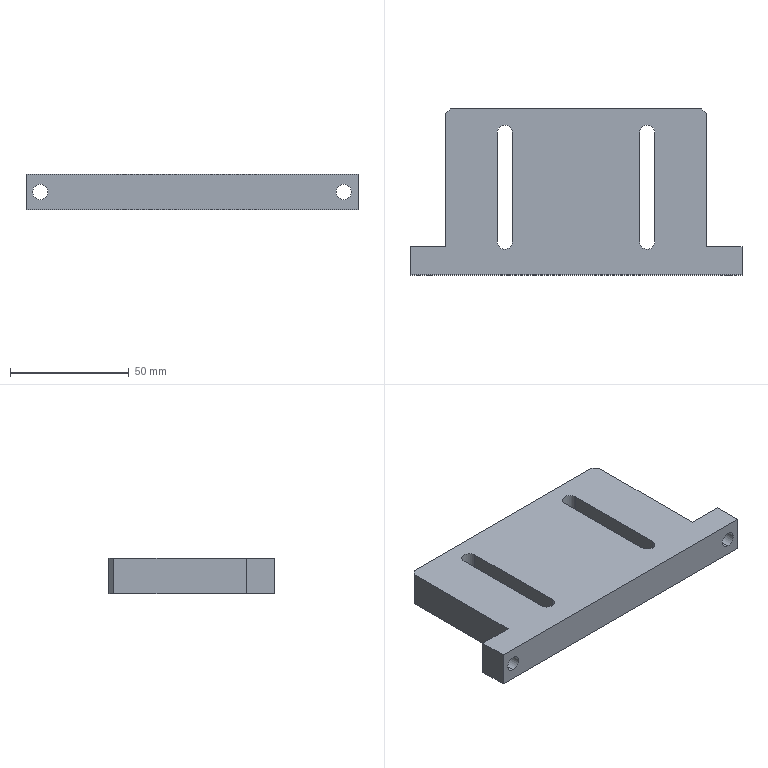Part | STEP file | 11-FG-S01011 | 1 solid | 24 faces | box 140 x 70 x 15 mm | volume 110078 mm3 | plane 16 | cylinder 8 | commonest cylinder face diameters 6.5 x8
STEP:
#1=CARTESIAN_POINT('',(64.,-35.,4.25));
#2=VERTEX_POINT('',#1);
#3=CARTESIAN_POINT('',(64.,-35.,10.75));
#4=VERTEX_POINT('',#3);
#5=CARTESIAN_POINT('',(64.,-35.,7.5));
#6=DIRECTION('',(0.,1.,0.));
#7=DIRECTION('',(0.,0.,1.));
#8=AXIS2_PLACEMENT_3D('',#5,#6,#7);
#9=CIRCLE('',#8,3.25);
#10=EDGE_CURVE('',#2,#4,#9,.T.);
#11=ORIENTED_EDGE('',*,*,#10,.F.);
#12=CARTESIAN_POINT('',(64.,-23.,4.25));
#13=VERTEX_POINT('',#12);
#14=CARTESIAN_POINT('',(64.,-41.,4.25));
#15=DIRECTION('',(0.,1.,0.));
#16=VECTOR('',#15,1000.);
#17=LINE('',#14,#16);
#18=EDGE_CURVE('',#2,#13,#17,.T.);
#19=ORIENTED_EDGE('',*,*,#18,.T.);
#20=CARTESIAN_POINT('',(64.,-23.,10.75));
#21=VERTEX_POINT('',#20);
#22=CARTESIAN_POINT('',(64.,-23.,7.5));
#23=DIRECTION('',(0.,1.,0.));
#24=DIRECTION('',(0.,0.,-1.));
#25=AXIS2_PLACEMENT_3D('',#22,#23,#24);
#26=CIRCLE('',#25,3.25);
#27=EDGE_CURVE('',#13,#21,#26,.T.);
#28=ORIENTED_EDGE('',*,*,#27,.T.);
#29=CARTESIAN_POINT('',(64.,-41.,10.75));
#30=DIRECTION('',(0.,1.,0.));
#31=VECTOR('',#30,1000.);
#32=LINE('',#29,#31);
#33=EDGE_CURVE('',#4,#21,#32,.T.);
#34=ORIENTED_EDGE('',*,*,#33,.F.);
#35=EDGE_LOOP('',(#11,#19,#28,#34));
#36=FACE_OUTER_BOUND('',#35,.T.);
#37=CARTESIAN_POINT('',(64.,-41.,7.5));
#38=DIRECTION('',(0.,1.,0.));
#39=DIRECTION('',(0.,0.,1.));
#40=AXIS2_PLACEMENT_3D('',#37,#38,#39);
#41=CYLINDRICAL_SURFACE('',#40,3.25);
#42=ADVANCED_FACE('',(#36),#41,.F.);
#43=CARTESIAN_POINT('',(-64.,-35.,4.25));
#44=VERTEX_POINT('',#43);
#45=CARTESIAN_POINT('',(-64.,-35.,10.75));
#46=VERTEX_POINT('',#45);
#47=CARTESIAN_POINT('',(-64.,-35.,7.5));
#48=DIRECTION('',(0.,1.,0.));
#49=DIRECTION('',(0.,0.,1.));
#50=AXIS2_PLACEMENT_3D('',#47,#48,#49);
#51=CIRCLE('',#50,3.25);
#52=EDGE_CURVE('',#44,#46,#51,.T.);
#53=ORIENTED_EDGE('',*,*,#52,.F.);
#54=CARTESIAN_POINT('',(-64.,-23.,4.25));
#55=VERTEX_POINT('',#54);
#56=CARTESIAN_POINT('',(-64.,-41.,4.25));
#57=DIRECTION('',(0.,1.,0.));
#58=VECTOR('',#57,1000.);
#59=LINE('',#56,#58);
#60=EDGE_CURVE('',#44,#55,#59,.T.);
#61=ORIENTED_EDGE('',*,*,#60,.T.);
#62=CARTESIAN_POINT('',(-64.,-23.,10.75));
#63=VERTEX_POINT('',#62);
#64=CARTESIAN_POINT('',(-64.,-23.,7.5));
#65=DIRECTION('',(0.,1.,0.));
#66=DIRECTION('',(0.,0.,1.));
#67=AXIS2_PLACEMENT_3D('',#64,#65,#66);
#68=CIRCLE('',#67,3.25);
#69=EDGE_CURVE('',#55,#63,#68,.T.);
#70=ORIENTED_EDGE('',*,*,#69,.T.);
#71=CARTESIAN_POINT('',(-64.,-41.,10.75));
#72=DIRECTION('',(0.,1.,0.));
#73=VECTOR('',#72,1000.);
#74=LINE('',#71,#73);
#75=EDGE_CURVE('',#46,#63,#74,.T.);
#76=ORIENTED_EDGE('',*,*,#75,.F.);
#77=EDGE_LOOP('',(#53,#61,#70,#76));
#78=FACE_OUTER_BOUND('',#77,.T.);
#79=CARTESIAN_POINT('',(-64.,-41.,7.5));
#80=DIRECTION('',(0.,1.,0.));
#81=DIRECTION('',(0.,0.,1.));
#82=AXIS2_PLACEMENT_3D('',#79,#80,#81);
#83=CYLINDRICAL_SURFACE('',#82,3.25);
#84=ADVANCED_FACE('',(#78),#83,.F.);
#85=CARTESIAN_POINT('',(-55.,33.,15.));
#86=VERTEX_POINT('',#85);
#87=CARTESIAN_POINT('',(-55.,-23.,15.));
#88=VERTEX_POINT('',#87);
#89=CARTESIAN_POINT('',(-55.,35.,15.));
#90=DIRECTION('',(0.,-1.,0.));
#91=VECTOR('',#90,1000.);
#92=LINE('',#89,#91);
#93=EDGE_CURVE('',#86,#88,#92,.T.);
#94=ORIENTED_EDGE('',*,*,#93,.F.);
#95=CARTESIAN_POINT('',(-55.,33.,0.));
#96=VERTEX_POINT('',#95);
#97=CARTESIAN_POINT('',(-55.,33.,15.));
#98=DIRECTION('',(0.,0.,-1.));
#99=VECTOR('',#98,1000.);
#100=LINE('',#97,#99);
#101=EDGE_CURVE('',#86,#96,#100,.T.);
#102=ORIENTED_EDGE('',*,*,#101,.T.);
#103=CARTESIAN_POINT('',(-55.,-23.,0.));
#104=VERTEX_POINT('',#103);
#105=CARTESIAN_POINT('',(-55.,35.,0.));
#106=DIRECTION('',(0.,-1.,0.));
#107=VECTOR('',#106,1000.);
#108=LINE('',#105,#107);
#109=EDGE_CURVE('',#96,#104,#108,.T.);
#110=ORIENTED_EDGE('',*,*,#109,.T.);
#111=CARTESIAN_POINT('',(-55.,-23.,34.209));
#112=DIRECTION('',(0.,0.,-1.));
#113=VECTOR('',#112,1000.);
#114=LINE('',#111,#113);
#115=EDGE_CURVE('',#88,#104,#114,.T.);
#116=ORIENTED_EDGE('',*,*,#115,.F.);
#117=EDGE_LOOP('',(#94,#102,#110,#116));
#118=FACE_OUTER_BOUND('',#117,.T.);
#119=CARTESIAN_POINT('',(-55.,35.,15.));
#120=DIRECTION('',(1.,0.,0.));
#121=DIRECTION('',(0.,0.,-1.));
#122=AXIS2_PLACEMENT_3D('',#119,#120,#121);
#123=PLANE('',#122);
#124=ADVANCED_FACE('',(#118),#123,.F.);
#125=CARTESIAN_POINT('',(55.,-23.,0.));
#126=VERTEX_POINT('',#125);
#127=CARTESIAN_POINT('',(55.,33.,0.));
#128=VERTEX_POINT('',#127);
#129=CARTESIAN_POINT('',(55.,35.,0.));
#130=DIRECTION('',(0.,1.,0.));
#131=VECTOR('',#130,1000.);
#132=LINE('',#129,#131);
#133=EDGE_CURVE('',#126,#128,#132,.T.);
#134=ORIENTED_EDGE('',*,*,#133,.T.);
#135=CARTESIAN_POINT('',(55.,33.,15.));
#136=VERTEX_POINT('',#135);
#137=CARTESIAN_POINT('',(55.,33.,15.));
#138=DIRECTION('',(0.,0.,1.));
#139=VECTOR('',#138,1000.);
#140=LINE('',#137,#139);
#141=EDGE_CURVE('',#128,#136,#140,.T.);
#142=ORIENTED_EDGE('',*,*,#141,.T.);
#143=CARTESIAN_POINT('',(55.,-23.,15.));
#144=VERTEX_POINT('',#143);
#145=CARTESIAN_POINT('',(55.,35.,15.));
#146=DIRECTION('',(0.,1.,0.));
#147=VECTOR('',#146,1000.);
#148=LINE('',#145,#147);
#149=EDGE_CURVE('',#144,#136,#148,.T.);
#150=ORIENTED_EDGE('',*,*,#149,.F.);
#151=CARTESIAN_POINT('',(55.,-23.,34.209));
#152=DIRECTION('',(0.,0.,-1.));
#153=VECTOR('',#152,1000.);
#154=LINE('',#151,#153);
#155=EDGE_CURVE('',#144,#126,#154,.T.);
#156=ORIENTED_EDGE('',*,*,#155,.T.);
#157=EDGE_LOOP('',(#134,#142,#150,#156));
#158=FACE_OUTER_BOUND('',#157,.T.);
#159=CARTESIAN_POINT('',(55.,35.,15.));
#160=DIRECTION('',(-1.,0.,0.));
#161=DIRECTION('',(0.,-1.,0.));
#162=AXIS2_PLACEMENT_3D('',#159,#160,#161);
#163=PLANE('',#162);
#164=ADVANCED_FACE('',(#158),#163,.F.);
#165=CARTESIAN_POINT('',(53.,35.,15.));
#166=VERTEX_POINT('',#165);
#167=CARTESIAN_POINT('',(-53.,35.,15.));
#168=VERTEX_POINT('',#167);
#169=CARTESIAN_POINT('',(-55.,35.,15.));
#170=DIRECTION('',(-1.,0.,0.));
#171=VECTOR('',#170,1000.);
#172=LINE('',#169,#171);
#173=EDGE_CURVE('',#166,#168,#172,.T.);
#174=ORIENTED_EDGE('',*,*,#173,.F.);
#175=CARTESIAN_POINT('',(53.,35.,0.));
#176=VERTEX_POINT('',#175);
#177=CARTESIAN_POINT('',(53.,35.,15.));
#178=DIRECTION('',(0.,0.,-1.));
#179=VECTOR('',#178,1000.);
#180=LINE('',#177,#179);
#181=EDGE_CURVE('',#166,#176,#180,.T.);
#182=ORIENTED_EDGE('',*,*,#181,.T.);
#183=CARTESIAN_POINT('',(-53.,35.,0.));
#184=VERTEX_POINT('',#183);
#185=CARTESIAN_POINT('',(-55.,35.,0.));
#186=DIRECTION('',(-1.,0.,0.));
#187=VECTOR('',#186,1000.);
#188=LINE('',#185,#187);
#189=EDGE_CURVE('',#176,#184,#188,.T.);
#190=ORIENTED_EDGE('',*,*,#189,.T.);
#191=CARTESIAN_POINT('',(-53.,35.,15.));
#192=DIRECTION('',(0.,0.,1.));
#193=VECTOR('',#192,1000.);
#194=LINE('',#191,#193);
#195=EDGE_CURVE('',#184,#168,#194,.T.);
#196=ORIENTED_EDGE('',*,*,#195,.T.);
#197=EDGE_LOOP('',(#174,#182,#190,#196));
#198=FACE_OUTER_BOUND('',#197,.T.);
#199=CARTESIAN_POINT('',(-55.,35.,15.));
#200=DIRECTION('',(0.,-1.,0.));
#201=DIRECTION('',(0.,0.,-1.));
#202=AXIS2_PLACEMENT_3D('',#199,#200,#201);
#203=PLANE('',#202);
#204=ADVANCED_FACE('',(#198),#203,.F.);
#205=CARTESIAN_POINT('',(64.,-35.,7.5));
#206=DIRECTION('',(0.,1.,0.));
#207=DIRECTION('',(0.,0.,1.));
#208=AXIS2_PLACEMENT_3D('',#205,#206,#207);
#209=CIRCLE('',#208,3.25);
#210=EDGE_CURVE('',#4,#2,#209,.T.);
#211=ORIENTED_EDGE('',*,*,#210,.T.);
#212=ORIENTED_EDGE('',*,*,#10,.T.);
#213=EDGE_LOOP('',(#211,#212));
#214=FACE_BOUND('',#213,.T.);
#215=CARTESIAN_POINT('',(-64.,-35.,7.5));
#216=DIRECTION('',(0.,1.,0.));
#217=DIRECTION('',(0.,0.,1.));
#218=AXIS2_PLACEMENT_3D('',#215,#216,#217);
#219=CIRCLE('',#218,3.25);
#220=EDGE_CURVE('',#46,#44,#219,.T.);
#221=ORIENTED_EDGE('',*,*,#220,.T.);
#222=ORIENTED_EDGE('',*,*,#52,.T.);
#223=EDGE_LOOP('',(#221,#222));
#224=FACE_BOUND('',#223,.T.);
#225=CARTESIAN_POINT('',(-70.,-35.,0.));
#226=VERTEX_POINT('',#225);
#227=CARTESIAN_POINT('',(70.,-35.,0.));
#228=VERTEX_POINT('',#227);
#229=CARTESIAN_POINT('',(-55.,-35.,0.));
#230=DIRECTION('',(1.,0.,0.));
#231=VECTOR('',#230,1000.);
#232=LINE('',#229,#231);
#233=EDGE_CURVE('',#226,#228,#232,.T.);
#234=ORIENTED_EDGE('',*,*,#233,.T.);
#235=CARTESIAN_POINT('',(70.,-35.,15.));
#236=VERTEX_POINT('',#235);
#237=CARTESIAN_POINT('',(70.,-35.,34.209));
#238=DIRECTION('',(0.,0.,-1.));
#239=VECTOR('',#238,1000.);
#240=LINE('',#237,#239);
#241=EDGE_CURVE('',#236,#228,#240,.T.);
#242=ORIENTED_EDGE('',*,*,#241,.F.);
#243=CARTESIAN_POINT('',(-70.,-35.,15.));
#244=VERTEX_POINT('',#243);
#245=CARTESIAN_POINT('',(-55.,-35.,15.));
#246=DIRECTION('',(1.,0.,0.));
#247=VECTOR('',#246,1000.);
#248=LINE('',#245,#247);
#249=EDGE_CURVE('',#244,#236,#248,.T.);
#250=ORIENTED_EDGE('',*,*,#249,.F.);
#251=CARTESIAN_POINT('',(-70.,-35.,34.209));
#252=DIRECTION('',(0.,0.,-1.));
#253=VECTOR('',#252,1000.);
#254=LINE('',#251,#253);
#255=EDGE_CURVE('',#244,#226,#254,.T.);
#256=ORIENTED_EDGE('',*,*,#255,.T.);
#257=EDGE_LOOP('',(#234,#242,#250,#256));
#258=FACE_OUTER_BOUND('',#257,.T.);
#259=CARTESIAN_POINT('',(-55.,-35.,15.));
#260=DIRECTION('',(0.,1.,0.));
#261=DIRECTION('',(0.,0.,1.));
#262=AXIS2_PLACEMENT_3D('',#259,#260,#261);
#263=PLANE('',#262);
#264=ADVANCED_FACE('',(#214,#224,#258),#263,.F.);
#265=CARTESIAN_POINT('',(-26.75,25.,15.));
#266=VERTEX_POINT('',#265);
#267=CARTESIAN_POINT('',(-33.25,25.,15.));
#268=VERTEX_POINT('',#267);
#269=CARTESIAN_POINT('',(-30.,25.,15.));
#270=DIRECTION('',(0.,0.,1.));
#271=DIRECTION('',(1.,0.,0.));
#272=AXIS2_PLACEMENT_3D('',#269,#270,#271);
#273=CIRCLE('',#272,3.25);
#274=EDGE_CURVE('',#266,#268,#273,.T.);
#275=ORIENTED_EDGE('',*,*,#274,.F.);
#276=CARTESIAN_POINT('',(-26.75,-21.,15.));
#277=VERTEX_POINT('',#276);
#278=CARTESIAN_POINT('',(-26.75,0.,15.));
#279=DIRECTION('',(0.,1.,0.));
#280=VECTOR('',#279,1000.);
#281=LINE('',#278,#280);
#282=EDGE_CURVE('',#277,#266,#281,.T.);
#283=ORIENTED_EDGE('',*,*,#282,.F.);
#284=CARTESIAN_POINT('',(-33.25,-21.,15.));
#285=VERTEX_POINT('',#284);
#286=CARTESIAN_POINT('',(-30.,-21.,15.));
#287=DIRECTION('',(0.,0.,1.));
#288=DIRECTION('',(1.,0.,0.));
#289=AXIS2_PLACEMENT_3D('',#286,#287,#288);
#290=CIRCLE('',#289,3.25);
#291=EDGE_CURVE('',#285,#277,#290,.T.);
#292=ORIENTED_EDGE('',*,*,#291,.F.);
#293=CARTESIAN_POINT('',(-33.25,0.,15.));
#294=DIRECTION('',(0.,-1.,0.));
#295=VECTOR('',#294,1000.);
#296=LINE('',#293,#295);
#297=EDGE_CURVE('',#268,#285,#296,.T.);
#298=ORIENTED_EDGE('',*,*,#297,.F.);
#299=EDGE_LOOP('',(#275,#283,#292,#298));
#300=FACE_BOUND('',#299,.T.);
#301=CARTESIAN_POINT('',(33.25,25.,15.));
#302=VERTEX_POINT('',#301);
#303=CARTESIAN_POINT('',(26.75,25.,15.));
#304=VERTEX_POINT('',#303);
#305=CARTESIAN_POINT('',(30.,25.,15.));
#306=DIRECTION('',(0.,0.,1.));
#307=DIRECTION('',(1.,0.,0.));
#308=AXIS2_PLACEMENT_3D('',#305,#306,#307);
#309=CIRCLE('',#308,3.25);
#310=EDGE_CURVE('',#302,#304,#309,.T.);
#311=ORIENTED_EDGE('',*,*,#310,.F.);
#312=CARTESIAN_POINT('',(33.25,-21.,15.));
#313=VERTEX_POINT('',#312);
#314=CARTESIAN_POINT('',(33.25,0.,15.));
#315=DIRECTION('',(0.,1.,0.));
#316=VECTOR('',#315,1000.);
#317=LINE('',#314,#316);
#318=EDGE_CURVE('',#313,#302,#317,.T.);
#319=ORIENTED_EDGE('',*,*,#318,.F.);
#320=CARTESIAN_POINT('',(26.75,-21.,15.));
#321=VERTEX_POINT('',#320);
#322=CARTESIAN_POINT('',(30.,-21.,15.));
#323=DIRECTION('',(0.,0.,1.));
#324=DIRECTION('',(1.,0.,0.));
#325=AXIS2_PLACEMENT_3D('',#322,#323,#324);
#326=CIRCLE('',#325,3.25);
#327=EDGE_CURVE('',#321,#313,#326,.T.);
#328=ORIENTED_EDGE('',*,*,#327,.F.);
#329=CARTESIAN_POINT('',(26.75,0.,15.));
#330=DIRECTION('',(0.,-1.,0.));
#331=VECTOR('',#330,1000.);
#332=LINE('',#329,#331);
#333=EDGE_CURVE('',#304,#321,#332,.T.);
#334=ORIENTED_EDGE('',*,*,#333,.F.);
#335=EDGE_LOOP('',(#311,#319,#328,#334));
#336=FACE_BOUND('',#335,.T.);
#337=ORIENTED_EDGE('',*,*,#149,.T.);
#338=CARTESIAN_POINT('',(44.,44.,15.));
#339=DIRECTION('',(-0.7071,0.7071,0.));
#340=VECTOR('',#339,1000.);
#341=LINE('',#338,#340);
#342=EDGE_CURVE('',#136,#166,#341,.T.);
#343=ORIENTED_EDGE('',*,*,#342,.T.);
#344=ORIENTED_EDGE('',*,*,#173,.T.);
#345=CARTESIAN_POINT('',(-44.,44.,15.));
#346=DIRECTION('',(-0.7071,-0.7071,0.));
#347=VECTOR('',#346,1000.);
#348=LINE('',#345,#347);
#349=EDGE_CURVE('',#168,#86,#348,.T.);
#350=ORIENTED_EDGE('',*,*,#349,.T.);
#351=ORIENTED_EDGE('',*,*,#93,.T.);
#352=CARTESIAN_POINT('',(-70.,-23.,15.));
#353=VERTEX_POINT('',#352);
#354=CARTESIAN_POINT('',(-55.,-23.,15.));
#355=DIRECTION('',(1.,0.,0.));
#356=VECTOR('',#355,1000.);
#357=LINE('',#354,#356);
#358=EDGE_CURVE('',#353,#88,#357,.T.);
#359=ORIENTED_EDGE('',*,*,#358,.F.);
#360=CARTESIAN_POINT('',(-70.,-35.,15.));
#361=DIRECTION('',(0.,1.,0.));
#362=VECTOR('',#361,1000.);
#363=LINE('',#360,#362);
#364=EDGE_CURVE('',#244,#353,#363,.T.);
#365=ORIENTED_EDGE('',*,*,#364,.F.);
#366=ORIENTED_EDGE('',*,*,#249,.T.);
#367=CARTESIAN_POINT('',(70.,-23.,15.));
#368=VERTEX_POINT('',#367);
#369=CARTESIAN_POINT('',(70.,-35.,15.));
#370=DIRECTION('',(0.,-1.,0.));
#371=VECTOR('',#370,1000.);
#372=LINE('',#369,#371);
#373=EDGE_CURVE('',#368,#236,#372,.T.);
#374=ORIENTED_EDGE('',*,*,#373,.F.);
#375=CARTESIAN_POINT('',(55.,-23.,15.));
#376=DIRECTION('',(1.,0.,0.));
#377=VECTOR('',#376,1000.);
#378=LINE('',#375,#377);
#379=EDGE_CURVE('',#144,#368,#378,.T.);
#380=ORIENTED_EDGE('',*,*,#379,.F.);
#381=EDGE_LOOP('',(#337,#343,#344,#350,#351,#359,#365,#366,#374,#380));
#382=FACE_OUTER_BOUND('',#381,.T.);
#383=CARTESIAN_POINT('',(0.,0.,15.));
#384=DIRECTION('',(0.,0.,1.));
#385=DIRECTION('',(1.,0.,0.));
#386=AXIS2_PLACEMENT_3D('',#383,#384,#385);
#387=PLANE('',#386);
#388=ADVANCED_FACE('',(#300,#336,#382),#387,.T.);
#389=CARTESIAN_POINT('',(-26.75,25.,0.));
#390=VERTEX_POINT('',#389);
#391=CARTESIAN_POINT('',(-26.75,-21.,0.));
#392=VERTEX_POINT('',#391);
#393=CARTESIAN_POINT('',(-26.75,25.,0.));
#394=DIRECTION('',(0.,-1.,0.));
#395=VECTOR('',#394,1000.);
#396=LINE('',#393,#395);
#397=EDGE_CURVE('',#390,#392,#396,.T.);
#398=ORIENTED_EDGE('',*,*,#397,.F.);
#399=CARTESIAN_POINT('',(-33.25,25.,0.));
#400=VERTEX_POINT('',#399);
#401=CARTESIAN_POINT('',(-30.,25.,0.));
#402=DIRECTION('',(0.,0.,-1.));
#403=DIRECTION('',(-1.,0.,0.));
#404=AXIS2_PLACEMENT_3D('',#401,#402,#403);
#405=CIRCLE('',#404,3.25);
#406=EDGE_CURVE('',#400,#390,#405,.T.);
#407=ORIENTED_EDGE('',*,*,#406,.F.);
#408=CARTESIAN_POINT('',(-33.25,-21.,0.));
#409=VERTEX_POINT('',#408);
#410=CARTESIAN_POINT('',(-33.25,25.,0.));
#411=DIRECTION('',(0.,1.,0.));
#412=VECTOR('',#411,1000.);
#413=LINE('',#410,#412);
#414=EDGE_CURVE('',#409,#400,#413,.T.);
#415=ORIENTED_EDGE('',*,*,#414,.F.);
#416=CARTESIAN_POINT('',(-30.,-21.,0.));
#417=DIRECTION('',(0.,0.,-1.));
#418=DIRECTION('',(-1.,0.,0.));
#419=AXIS2_PLACEMENT_3D('',#416,#417,#418);
#420=CIRCLE('',#419,3.25);
#421=EDGE_CURVE('',#392,#409,#420,.T.);
#422=ORIENTED_EDGE('',*,*,#421,.F.);
#423=EDGE_LOOP('',(#398,#407,#415,#422));
#424=FACE_BOUND('',#423,.T.);
#425=CARTESIAN_POINT('',(33.25,25.,0.));
#426=VERTEX_POINT('',#425);
#427=CARTESIAN_POINT('',(33.25,-21.,0.));
#428=VERTEX_POINT('',#427);
#429=CARTESIAN_POINT('',(33.25,25.,0.));
#430=DIRECTION('',(0.,-1.,0.));
#431=VECTOR('',#430,1000.);
#432=LINE('',#429,#431);
#433=EDGE_CURVE('',#426,#428,#432,.T.);
#434=ORIENTED_EDGE('',*,*,#433,.F.);
#435=CARTESIAN_POINT('',(26.75,25.,0.));
#436=VERTEX_POINT('',#435);
#437=CARTESIAN_POINT('',(30.,25.,0.));
#438=DIRECTION('',(0.,0.,-1.));
#439=DIRECTION('',(-1.,0.,0.));
#440=AXIS2_PLACEMENT_3D('',#437,#438,#439);
#441=CIRCLE('',#440,3.25);
#442=EDGE_CURVE('',#436,#426,#441,.T.);
#443=ORIENTED_EDGE('',*,*,#442,.F.);
#444=CARTESIAN_POINT('',(26.75,-21.,0.));
#445=VERTEX_POINT('',#444);
#446=CARTESIAN_POINT('',(26.75,25.,0.));
#447=DIRECTION('',(0.,1.,0.));
#448=VECTOR('',#447,1000.);
#449=LINE('',#446,#448);
#450=EDGE_CURVE('',#445,#436,#449,.T.);
#451=ORIENTED_EDGE('',*,*,#450,.F.);
#452=CARTESIAN_POINT('',(30.,-21.,0.));
#453=DIRECTION('',(0.,0.,-1.));
#454=DIRECTION('',(-1.,0.,0.));
#455=AXIS2_PLACEMENT_3D('',#452,#453,#454);
#456=CIRCLE('',#455,3.25);
#457=EDGE_CURVE('',#428,#445,#456,.T.);
#458=ORIENTED_EDGE('',*,*,#457,.F.);
#459=EDGE_LOOP('',(#434,#443,#451,#458));
#460=FACE_BOUND('',#459,.T.);
#461=ORIENTED_EDGE('',*,*,#189,.F.);
#462=CARTESIAN_POINT('',(53.,35.,0.));
#463=DIRECTION('',(0.7071,-0.7071,0.));
#464=VECTOR('',#463,1000.);
#465=LINE('',#462,#464);
#466=EDGE_CURVE('',#176,#128,#465,.T.);
#467=ORIENTED_EDGE('',*,*,#466,.T.);
#468=ORIENTED_EDGE('',*,*,#133,.F.);
#469=CARTESIAN_POINT('',(70.,-23.,0.));
#470=VERTEX_POINT('',#469);
#471=CARTESIAN_POINT('',(55.,-23.,0.));
#472=DIRECTION('',(1.,0.,0.));
#473=VECTOR('',#472,1000.);
#474=LINE('',#471,#473);
#475=EDGE_CURVE('',#126,#470,#474,.T.);
#476=ORIENTED_EDGE('',*,*,#475,.T.);
#477=CARTESIAN_POINT('',(70.,-35.,0.));
#478=DIRECTION('',(0.,-1.,0.));
#479=VECTOR('',#478,1000.);
#480=LINE('',#477,#479);
#481=EDGE_CURVE('',#470,#228,#480,.T.);
#482=ORIENTED_EDGE('',*,*,#481,.T.);
#483=ORIENTED_EDGE('',*,*,#233,.F.);
#484=CARTESIAN_POINT('',(-70.,-23.,0.));
#485=VERTEX_POINT('',#484);
#486=CARTESIAN_POINT('',(-70.,-35.,0.));
#487=DIRECTION('',(0.,1.,0.));
#488=VECTOR('',#487,1000.);
#489=LINE('',#486,#488);
#490=EDGE_CURVE('',#226,#485,#489,.T.);
#491=ORIENTED_EDGE('',*,*,#490,.T.);
#492=CARTESIAN_POINT('',(-55.,-23.,0.));
#493=DIRECTION('',(1.,0.,0.));
#494=VECTOR('',#493,1000.);
#495=LINE('',#492,#494);
#496=EDGE_CURVE('',#485,#104,#495,.T.);
#497=ORIENTED_EDGE('',*,*,#496,.T.);
#498=ORIENTED_EDGE('',*,*,#109,.F.);
#499=CARTESIAN_POINT('',(-55.,33.,0.));
#500=DIRECTION('',(0.7071,0.7071,0.));
#501=VECTOR('',#500,1000.);
#502=LINE('',#499,#501);
#503=EDGE_CURVE('',#96,#184,#502,.T.);
#504=ORIENTED_EDGE('',*,*,#503,.T.);
#505=EDGE_LOOP('',(#461,#467,#468,#476,#482,#483,#491,#497,#498,#504));
#506=FACE_OUTER_BOUND('',#505,.T.);
#507=CARTESIAN_POINT('',(0.,0.,0.));
#508=DIRECTION('',(0.,0.,1.));
#509=DIRECTION('',(1.,0.,0.));
#510=AXIS2_PLACEMENT_3D('',#507,#508,#509);
#511=PLANE('',#510);
#512=ADVANCED_FACE('',(#424,#460,#506),#511,.F.);
#513=CARTESIAN_POINT('',(64.,-23.,7.5));
#514=DIRECTION('',(0.,1.,0.));
#515=DIRECTION('',(0.,0.,-1.));
#516=AXIS2_PLACEMENT_3D('',#513,#514,#515);
#517=CIRCLE('',#516,3.25);
#518=EDGE_CURVE('',#21,#13,#517,.T.);
#519=ORIENTED_EDGE('',*,*,#518,.F.);
#520=ORIENTED_EDGE('',*,*,#27,.F.);
#521=EDGE_LOOP('',(#519,#520));
#522=FACE_BOUND('',#521,.T.);
#523=ORIENTED_EDGE('',*,*,#155,.F.);
#524=ORIENTED_EDGE('',*,*,#379,.T.);
#525=CARTESIAN_POINT('',(70.,-23.,34.209));
#526=DIRECTION('',(0.,0.,-1.));
#527=VECTOR('',#526,1000.);
#528=LINE('',#525,#527);
#529=EDGE_CURVE('',#368,#470,#528,.T.);
#530=ORIENTED_EDGE('',*,*,#529,.T.);
#531=ORIENTED_EDGE('',*,*,#475,.F.);
#532=EDGE_LOOP('',(#523,#524,#530,#531));
#533=FACE_OUTER_BOUND('',#532,.T.);
#534=CARTESIAN_POINT('',(55.,-23.,34.209));
#535=DIRECTION('',(0.,1.,0.));
#536=DIRECTION('',(0.,0.,1.));
#537=AXIS2_PLACEMENT_3D('',#534,#535,#536);
#538=PLANE('',#537);
#539=ADVANCED_FACE('',(#522,#533),#538,.T.);
#540=ORIENTED_EDGE('',*,*,#529,.F.);
#541=ORIENTED_EDGE('',*,*,#373,.T.);
#542=ORIENTED_EDGE('',*,*,#241,.T.);
#543=ORIENTED_EDGE('',*,*,#481,.F.);
#544=EDGE_LOOP('',(#540,#541,#542,#543));
#545=FACE_OUTER_BOUND('',#544,.T.);
#546=CARTESIAN_POINT('',(70.,-35.,34.209));
#547=DIRECTION('',(1.,0.,0.));
#548=DIRECTION('',(0.,0.,-1.));
#549=AXIS2_PLACEMENT_3D('',#546,#547,#548);
#550=PLANE('',#549);
#551=ADVANCED_FACE('',(#545),#550,.T.);
#552=ORIENTED_EDGE('',*,*,#255,.F.);
#553=ORIENTED_EDGE('',*,*,#364,.T.);
#554=CARTESIAN_POINT('',(-70.,-23.,34.209));
#555=DIRECTION('',(0.,0.,-1.));
#556=VECTOR('',#555,1000.);
#557=LINE('',#554,#556);
#558=EDGE_CURVE('',#353,#485,#557,.T.);
#559=ORIENTED_EDGE('',*,*,#558,.T.);
#560=ORIENTED_EDGE('',*,*,#490,.F.);
#561=EDGE_LOOP('',(#552,#553,#559,#560));
#562=FACE_OUTER_BOUND('',#561,.T.);
#563=CARTESIAN_POINT('',(-70.,-35.,34.209));
#564=DIRECTION('',(-1.,0.,0.));
#565=DIRECTION('',(0.,0.,1.));
#566=AXIS2_PLACEMENT_3D('',#563,#564,#565);
#567=PLANE('',#566);
#568=ADVANCED_FACE('',(#562),#567,.T.);
#569=CARTESIAN_POINT('',(-64.,-23.,7.5));
#570=DIRECTION('',(0.,1.,0.));
#571=DIRECTION('',(0.,0.,1.));
#572=AXIS2_PLACEMENT_3D('',#569,#570,#571);
#573=CIRCLE('',#572,3.25);
#574=EDGE_CURVE('',#63,#55,#573,.T.);
#575=ORIENTED_EDGE('',*,*,#574,.F.);
#576=ORIENTED_EDGE('',*,*,#69,.F.);
#577=EDGE_LOOP('',(#575,#576));
#578=FACE_BOUND('',#577,.T.);
#579=ORIENTED_EDGE('',*,*,#558,.F.);
#580=ORIENTED_EDGE('',*,*,#358,.T.);
#581=ORIENTED_EDGE('',*,*,#115,.T.);
#582=ORIENTED_EDGE('',*,*,#496,.F.);
#583=EDGE_LOOP('',(#579,#580,#581,#582));
#584=FACE_OUTER_BOUND('',#583,.T.);
#585=CARTESIAN_POINT('',(-55.,-23.,34.209));
#586=DIRECTION('',(0.,1.,0.));
#587=DIRECTION('',(0.,0.,1.));
#588=AXIS2_PLACEMENT_3D('',#585,#586,#587);
#589=PLANE('',#588);
#590=ADVANCED_FACE('',(#578,#584),#589,.T.);
#591=ORIENTED_EDGE('',*,*,#60,.F.);
#592=ORIENTED_EDGE('',*,*,#220,.F.);
#593=ORIENTED_EDGE('',*,*,#75,.T.);
#594=ORIENTED_EDGE('',*,*,#574,.T.);
#595=EDGE_LOOP('',(#591,#592,#593,#594));
#596=FACE_OUTER_BOUND('',#595,.T.);
#597=CARTESIAN_POINT('',(-64.,-41.,7.5));
#598=DIRECTION('',(0.,1.,0.));
#599=DIRECTION('',(0.,0.,1.));
#600=AXIS2_PLACEMENT_3D('',#597,#598,#599);
#601=CYLINDRICAL_SURFACE('',#600,3.25);
#602=ADVANCED_FACE('',(#596),#601,.F.);
#603=ORIENTED_EDGE('',*,*,#18,.F.);
#604=ORIENTED_EDGE('',*,*,#210,.F.);
#605=ORIENTED_EDGE('',*,*,#33,.T.);
#606=ORIENTED_EDGE('',*,*,#518,.T.);
#607=EDGE_LOOP('',(#603,#604,#605,#606));
#608=FACE_OUTER_BOUND('',#607,.T.);
#609=CARTESIAN_POINT('',(64.,-41.,7.5));
#610=DIRECTION('',(0.,1.,0.));
#611=DIRECTION('',(0.,0.,1.));
#612=AXIS2_PLACEMENT_3D('',#609,#610,#611);
#613=CYLINDRICAL_SURFACE('',#612,3.25);
#614=ADVANCED_FACE('',(#608),#613,.F.);
#615=ORIENTED_EDGE('',*,*,#310,.T.);
#616=CARTESIAN_POINT('',(26.75,25.,45.));
#617=DIRECTION('',(0.,0.,-1.));
#618=VECTOR('',#617,1000.);
#619=LINE('',#616,#618);
#620=EDGE_CURVE('',#304,#436,#619,.T.);
#621=ORIENTED_EDGE('',*,*,#620,.T.);
#622=ORIENTED_EDGE('',*,*,#442,.T.);
#623=CARTESIAN_POINT('',(33.25,25.,45.));
#624=DIRECTION('',(0.,0.,-1.));
#625=VECTOR('',#624,1000.);
#626=LINE('',#623,#625);
#627=EDGE_CURVE('',#302,#426,#626,.T.);
#628=ORIENTED_EDGE('',*,*,#627,.F.);
#629=EDGE_LOOP('',(#615,#621,#622,#628));
#630=FACE_OUTER_BOUND('',#629,.T.);
#631=CARTESIAN_POINT('',(30.,25.,45.));
#632=DIRECTION('',(0.,0.,-1.));
#633=DIRECTION('',(-1.,0.,0.));
#634=AXIS2_PLACEMENT_3D('',#631,#632,#633);
#635=CYLINDRICAL_SURFACE('',#634,3.25);
#636=ADVANCED_FACE('',(#630),#635,.F.);
#637=ORIENTED_EDGE('',*,*,#333,.T.);
#638=CARTESIAN_POINT('',(26.75,-21.,45.));
#639=DIRECTION('',(0.,0.,-1.));
#640=VECTOR('',#639,1000.);
#641=LINE('',#638,#640);
#642=EDGE_CURVE('',#321,#445,#641,.T.);
#643=ORIENTED_EDGE('',*,*,#642,.T.);
#644=ORIENTED_EDGE('',*,*,#450,.T.);
#645=ORIENTED_EDGE('',*,*,#620,.F.);
#646=EDGE_LOOP('',(#637,#643,#644,#645));
#647=FACE_OUTER_BOUND('',#646,.T.);
#648=CARTESIAN_POINT('',(26.75,25.,45.));
#649=DIRECTION('',(-1.,0.,0.));
#650=DIRECTION('',(0.,0.,1.));
#651=AXIS2_PLACEMENT_3D('',#648,#649,#650);
#652=PLANE('',#651);
#653=ADVANCED_FACE('',(#647),#652,.F.);
#654=ORIENTED_EDGE('',*,*,#327,.T.);
#655=CARTESIAN_POINT('',(33.25,-21.,45.));
#656=DIRECTION('',(0.,0.,-1.));
#657=VECTOR('',#656,1000.);
#658=LINE('',#655,#657);
#659=EDGE_CURVE('',#313,#428,#658,.T.);
#660=ORIENTED_EDGE('',*,*,#659,.T.);
#661=ORIENTED_EDGE('',*,*,#457,.T.);
#662=ORIENTED_EDGE('',*,*,#642,.F.);
#663=EDGE_LOOP('',(#654,#660,#661,#662));
#664=FACE_OUTER_BOUND('',#663,.T.);
#665=CARTESIAN_POINT('',(30.,-21.,45.));
#666=DIRECTION('',(0.,0.,-1.));
#667=DIRECTION('',(-1.,0.,0.));
#668=AXIS2_PLACEMENT_3D('',#665,#666,#667);
#669=CYLINDRICAL_SURFACE('',#668,3.25);
#670=ADVANCED_FACE('',(#664),#669,.F.);
#671=ORIENTED_EDGE('',*,*,#318,.T.);
#672=ORIENTED_EDGE('',*,*,#627,.T.);
#673=ORIENTED_EDGE('',*,*,#433,.T.);
#674=ORIENTED_EDGE('',*,*,#659,.F.);
#675=EDGE_LOOP('',(#671,#672,#673,#674));
#676=FACE_OUTER_BOUND('',#675,.T.);
#677=CARTESIAN_POINT('',(33.25,25.,45.));
#678=DIRECTION('',(1.,0.,0.));
#679=DIRECTION('',(0.,1.,0.));
#680=AXIS2_PLACEMENT_3D('',#677,#678,#679);
#681=PLANE('',#680);
#682=ADVANCED_FACE('',(#676),#681,.F.);
#683=ORIENTED_EDGE('',*,*,#274,.T.);
#684=CARTESIAN_POINT('',(-33.25,25.,45.));
#685=DIRECTION('',(0.,0.,-1.));
#686=VECTOR('',#685,1000.);
#687=LINE('',#684,#686);
#688=EDGE_CURVE('',#268,#400,#687,.T.);
#689=ORIENTED_EDGE('',*,*,#688,.T.);
#690=ORIENTED_EDGE('',*,*,#406,.T.);
#691=CARTESIAN_POINT('',(-26.75,25.,45.));
#692=DIRECTION('',(0.,0.,-1.));
#693=VECTOR('',#692,1000.);
#694=LINE('',#691,#693);
#695=EDGE_CURVE('',#266,#390,#694,.T.);
#696=ORIENTED_EDGE('',*,*,#695,.F.);
#697=EDGE_LOOP('',(#683,#689,#690,#696));
#698=FACE_OUTER_BOUND('',#697,.T.);
#699=CARTESIAN_POINT('',(-30.,25.,45.));
#700=DIRECTION('',(0.,0.,-1.));
#701=DIRECTION('',(-1.,0.,0.));
#702=AXIS2_PLACEMENT_3D('',#699,#700,#701);
#703=CYLINDRICAL_SURFACE('',#702,3.25);
#704=ADVANCED_FACE('',(#698),#703,.F.);
#705=ORIENTED_EDGE('',*,*,#297,.T.);
#706=CARTESIAN_POINT('',(-33.25,-21.,45.));
#707=DIRECTION('',(0.,0.,-1.));
#708=VECTOR('',#707,1000.);
#709=LINE('',#706,#708);
#710=EDGE_CURVE('',#285,#409,#709,.T.);
#711=ORIENTED_EDGE('',*,*,#710,.T.);
#712=ORIENTED_EDGE('',*,*,#414,.T.);
#713=ORIENTED_EDGE('',*,*,#688,.F.);
#714=EDGE_LOOP('',(#705,#711,#712,#713));
#715=FACE_OUTER_BOUND('',#714,.T.);
#716=CARTESIAN_POINT('',(-33.25,25.,45.));
#717=DIRECTION('',(-1.,0.,0.));
#718=DIRECTION('',(0.,0.,1.));
#719=AXIS2_PLACEMENT_3D('',#716,#717,#718);
#720=PLANE('',#719);
#721=ADVANCED_FACE('',(#715),#720,.F.);
#722=ORIENTED_EDGE('',*,*,#291,.T.);
#723=CARTESIAN_POINT('',(-26.75,-21.,45.));
#724=DIRECTION('',(0.,0.,-1.));
#725=VECTOR('',#724,1000.);
#726=LINE('',#723,#725);
#727=EDGE_CURVE('',#277,#392,#726,.T.);
#728=ORIENTED_EDGE('',*,*,#727,.T.);
#729=ORIENTED_EDGE('',*,*,#421,.T.);
#730=ORIENTED_EDGE('',*,*,#710,.F.);
#731=EDGE_LOOP('',(#722,#728,#729,#730));
#732=FACE_OUTER_BOUND('',#731,.T.);
#733=CARTESIAN_POINT('',(-30.,-21.,45.));
#734=DIRECTION('',(0.,0.,-1.));
#735=DIRECTION('',(-1.,0.,0.));
#736=AXIS2_PLACEMENT_3D('',#733,#734,#735);
#737=CYLINDRICAL_SURFACE('',#736,3.25);
#738=ADVANCED_FACE('',(#732),#737,.F.);
#739=ORIENTED_EDGE('',*,*,#282,.T.);
#740=ORIENTED_EDGE('',*,*,#695,.T.);
#741=ORIENTED_EDGE('',*,*,#397,.T.);
#742=ORIENTED_EDGE('',*,*,#727,.F.);
#743=EDGE_LOOP('',(#739,#740,#741,#742));
#744=FACE_OUTER_BOUND('',#743,.T.);
#745=CARTESIAN_POINT('',(-26.75,25.,45.));
#746=DIRECTION('',(1.,0.,0.));
#747=DIRECTION('',(0.,1.,0.));
#748=AXIS2_PLACEMENT_3D('',#745,#746,#747);
#749=PLANE('',#748);
#750=ADVANCED_FACE('',(#744),#749,.F.);
#751=ORIENTED_EDGE('',*,*,#342,.F.);
#752=ORIENTED_EDGE('',*,*,#141,.F.);
#753=ORIENTED_EDGE('',*,*,#466,.F.);
#754=ORIENTED_EDGE('',*,*,#181,.F.);
#755=EDGE_LOOP('',(#751,#752,#753,#754));
#756=FACE_OUTER_BOUND('',#755,.T.);
#757=CARTESIAN_POINT('',(53.,35.,15.));
#758=DIRECTION('',(-0.7071,-0.7071,0.));
#759=DIRECTION('',(0.,0.,-1.));
#760=AXIS2_PLACEMENT_3D('',#757,#758,#759);
#761=PLANE('',#760);
#762=ADVANCED_FACE('',(#756),#761,.F.);
#763=ORIENTED_EDGE('',*,*,#349,.F.);
#764=ORIENTED_EDGE('',*,*,#195,.F.);
#765=ORIENTED_EDGE('',*,*,#503,.F.);
#766=ORIENTED_EDGE('',*,*,#101,.F.);
#767=EDGE_LOOP('',(#763,#764,#765,#766));
#768=FACE_OUTER_BOUND('',#767,.T.);
#769=CARTESIAN_POINT('',(-55.,33.,15.));
#770=DIRECTION('',(0.7071,-0.7071,0.));
#771=DIRECTION('',(0.,0.,-1.));
#772=AXIS2_PLACEMENT_3D('',#769,#770,#771);
#773=PLANE('',#772);
#774=ADVANCED_FACE('',(#768),#773,.F.);
#775=CLOSED_SHELL('',(#42,#84,#124,#164,#204,#264,#388,#512,#539,#551,#568,#590,#602,#614,#636,#653,#670,#682,#704,#721,#738,#750,#762,#774));
#776=MANIFOLD_SOLID_BREP('',#775);
#777=CARTESIAN_POINT('',(0.,0.,0.));
#778=DIRECTION('',(0.,0.,1.));
#779=DIRECTION('',(1.,0.,0.));
#780=AXIS2_PLACEMENT_3D('',#777,#778,#779);
#781=(LENGTH_UNIT()NAMED_UNIT(*)SI_UNIT(.MILLI.,.METRE.));
#782=UNCERTAINTY_MEASURE_WITH_UNIT(LENGTH_MEASURE(0.00001),#781,'','');
#783=(NAMED_UNIT(*)PLANE_ANGLE_UNIT()SI_UNIT($,.RADIAN.));
#784=(NAMED_UNIT(*)SI_UNIT($,.STERADIAN.)SOLID_ANGLE_UNIT());
#785=(GEOMETRIC_REPRESENTATION_CONTEXT(3)GLOBAL_UNCERTAINTY_ASSIGNED_CONTEXT((#782))GLOBAL_UNIT_ASSIGNED_CONTEXT((#781,#783,#784))REPRESENTATION_CONTEXT('',''));
#786=ADVANCED_BREP_SHAPE_REPRESENTATION('',(#776,#780),#785);